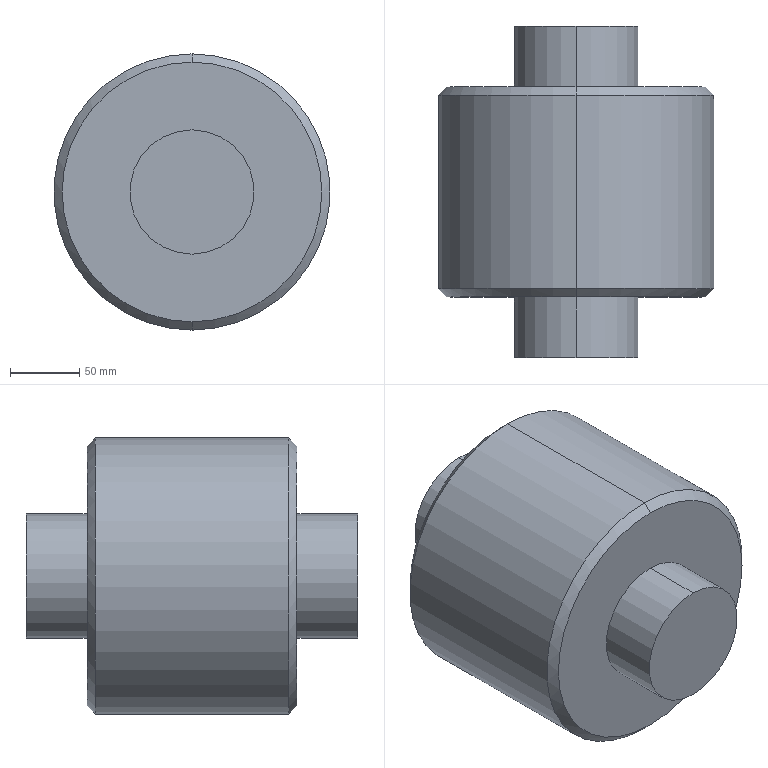Part | SolidWorks | features Chamfer 1, Extrusion 1, ICE 1 | 1 solid | 14 faces | box 200 x 240 x 200 mm | volume 5312886 mm3 | cylinder 6 | cone 4 | plane 4 | commonest cylinder face diameters 90 x4 200 x2
STEP:
#1=CARTESIAN_POINT('',(0.,196.,94.));
#2=VERTEX_POINT('',#1);
#3=CARTESIAN_POINT('',(0.,196.,-94.));
#4=VERTEX_POINT('',#3);
#5=CARTESIAN_POINT('',(0.,196.,0.));
#6=DIRECTION('',(0.,1.,0.));
#7=DIRECTION('',(0.,0.,1.));
#8=AXIS2_PLACEMENT_3D('',#5,#6,#7);
#9=CIRCLE('',#8,94.);
#10=EDGE_CURVE('',#2,#4,#9,.T.);
#11=ORIENTED_EDGE('',*,*,#10,.F.);
#12=CARTESIAN_POINT('',(0.,190.,100.));
#13=VERTEX_POINT('',#12);
#14=CARTESIAN_POINT('',(0.,196.,94.));
#15=DIRECTION('',(0.,-0.7071,0.7071));
#16=VECTOR('',#15,1000.);
#17=LINE('',#14,#16);
#18=EDGE_CURVE('',#2,#13,#17,.T.);
#19=ORIENTED_EDGE('',*,*,#18,.T.);
#20=CARTESIAN_POINT('',(0.,190.,-100.));
#21=VERTEX_POINT('',#20);
#22=CARTESIAN_POINT('',(0.,190.,0.));
#23=DIRECTION('',(0.,-1.,0.));
#24=DIRECTION('',(0.,0.,1.));
#25=AXIS2_PLACEMENT_3D('',#22,#23,#24);
#26=CIRCLE('',#25,100.);
#27=EDGE_CURVE('',#21,#13,#26,.T.);
#28=ORIENTED_EDGE('',*,*,#27,.F.);
#29=CARTESIAN_POINT('',(0.,196.,-94.));
#30=DIRECTION('',(0.,-0.7071,-0.7071));
#31=VECTOR('',#30,1000.);
#32=LINE('',#29,#31);
#33=EDGE_CURVE('',#4,#21,#32,.T.);
#34=ORIENTED_EDGE('',*,*,#33,.F.);
#35=EDGE_LOOP('',(#11,#19,#28,#34));
#36=FACE_OUTER_BOUND('',#35,.T.);
#37=CARTESIAN_POINT('',(0.,196.,0.));
#38=DIRECTION('',(0.,-1.,0.));
#39=DIRECTION('',(0.,0.,-1.));
#40=AXIS2_PLACEMENT_3D('',#37,#38,#39);
#41=CONICAL_SURFACE('',#40,94.,0.7854);
#42=ADVANCED_FACE('',(#36),#41,.T.);
#43=CARTESIAN_POINT('',(0.,44.,-94.));
#44=VERTEX_POINT('',#43);
#45=CARTESIAN_POINT('',(0.,44.,94.));
#46=VERTEX_POINT('',#45);
#47=CARTESIAN_POINT('',(0.,44.,0.));
#48=DIRECTION('',(0.,-1.,0.));
#49=DIRECTION('',(0.,0.,1.));
#50=AXIS2_PLACEMENT_3D('',#47,#48,#49);
#51=CIRCLE('',#50,94.);
#52=EDGE_CURVE('',#44,#46,#51,.T.);
#53=ORIENTED_EDGE('',*,*,#52,.F.);
#54=CARTESIAN_POINT('',(0.,50.,-100.));
#55=VERTEX_POINT('',#54);
#56=CARTESIAN_POINT('',(0.,50.,-100.));
#57=DIRECTION('',(0.,0.7071,-0.7071));
#58=VECTOR('',#57,1000.);
#59=LINE('',#56,#58);
#60=EDGE_CURVE('',#44,#55,#59,.T.);
#61=ORIENTED_EDGE('',*,*,#60,.T.);
#62=CARTESIAN_POINT('',(0.,50.,100.));
#63=VERTEX_POINT('',#62);
#64=CARTESIAN_POINT('',(0.,50.,0.));
#65=DIRECTION('',(0.,1.,0.));
#66=DIRECTION('',(0.,0.,1.));
#67=AXIS2_PLACEMENT_3D('',#64,#65,#66);
#68=CIRCLE('',#67,100.);
#69=EDGE_CURVE('',#63,#55,#68,.T.);
#70=ORIENTED_EDGE('',*,*,#69,.F.);
#71=CARTESIAN_POINT('',(0.,50.,100.));
#72=DIRECTION('',(0.,0.7071,0.7071));
#73=VECTOR('',#72,1000.);
#74=LINE('',#71,#73);
#75=EDGE_CURVE('',#46,#63,#74,.T.);
#76=ORIENTED_EDGE('',*,*,#75,.F.);
#77=EDGE_LOOP('',(#53,#61,#70,#76));
#78=FACE_OUTER_BOUND('',#77,.T.);
#79=CARTESIAN_POINT('',(0.,50.,0.));
#80=DIRECTION('',(0.,1.,0.));
#81=DIRECTION('',(0.,0.,1.));
#82=AXIS2_PLACEMENT_3D('',#79,#80,#81);
#83=CONICAL_SURFACE('',#82,100.,0.7854);
#84=ADVANCED_FACE('',(#78),#83,.T.);
#85=CARTESIAN_POINT('',(0.,240.,45.));
#86=VERTEX_POINT('',#85);
#87=CARTESIAN_POINT('',(0.,240.,-45.));
#88=VERTEX_POINT('',#87);
#89=CARTESIAN_POINT('',(0.,240.,0.));
#90=DIRECTION('',(0.,1.,0.));
#91=DIRECTION('',(0.,0.,1.));
#92=AXIS2_PLACEMENT_3D('',#89,#90,#91);
#93=CIRCLE('',#92,45.);
#94=EDGE_CURVE('',#86,#88,#93,.T.);
#95=ORIENTED_EDGE('',*,*,#94,.F.);
#96=CARTESIAN_POINT('',(0.,196.,45.));
#97=VERTEX_POINT('',#96);
#98=CARTESIAN_POINT('',(0.,240.,45.));
#99=DIRECTION('',(0.,-1.,0.));
#100=VECTOR('',#99,1000.);
#101=LINE('',#98,#100);
#102=EDGE_CURVE('',#86,#97,#101,.T.);
#103=ORIENTED_EDGE('',*,*,#102,.T.);
#104=CARTESIAN_POINT('',(0.,196.,-45.));
#105=VERTEX_POINT('',#104);
#106=CARTESIAN_POINT('',(0.,196.,0.));
#107=DIRECTION('',(0.,1.,0.));
#108=DIRECTION('',(0.,0.,1.));
#109=AXIS2_PLACEMENT_3D('',#106,#107,#108);
#110=CIRCLE('',#109,45.);
#111=EDGE_CURVE('',#97,#105,#110,.T.);
#112=ORIENTED_EDGE('',*,*,#111,.T.);
#113=CARTESIAN_POINT('',(0.,240.,-45.));
#114=DIRECTION('',(0.,-1.,0.));
#115=VECTOR('',#114,1000.);
#116=LINE('',#113,#115);
#117=EDGE_CURVE('',#88,#105,#116,.T.);
#118=ORIENTED_EDGE('',*,*,#117,.F.);
#119=EDGE_LOOP('',(#95,#103,#112,#118));
#120=FACE_OUTER_BOUND('',#119,.T.);
#121=CARTESIAN_POINT('',(0.,240.,0.));
#122=DIRECTION('',(0.,-1.,0.));
#123=DIRECTION('',(0.,0.,-1.));
#124=AXIS2_PLACEMENT_3D('',#121,#122,#123);
#125=CYLINDRICAL_SURFACE('',#124,45.);
#126=ADVANCED_FACE('',(#120),#125,.T.);
#127=ORIENTED_EDGE('',*,*,#69,.T.);
#128=CARTESIAN_POINT('',(0.,44.,-100.));
#129=DIRECTION('',(0.,1.,0.));
#130=VECTOR('',#129,1000.);
#131=LINE('',#128,#130);
#132=EDGE_CURVE('',#55,#21,#131,.T.);
#133=ORIENTED_EDGE('',*,*,#132,.T.);
#134=ORIENTED_EDGE('',*,*,#27,.T.);
#135=CARTESIAN_POINT('',(0.,44.,100.));
#136=DIRECTION('',(0.,1.,0.));
#137=VECTOR('',#136,1000.);
#138=LINE('',#135,#137);
#139=EDGE_CURVE('',#63,#13,#138,.T.);
#140=ORIENTED_EDGE('',*,*,#139,.F.);
#141=EDGE_LOOP('',(#127,#133,#134,#140));
#142=FACE_OUTER_BOUND('',#141,.T.);
#143=CARTESIAN_POINT('',(0.,44.,0.));
#144=DIRECTION('',(0.,1.,0.));
#145=DIRECTION('',(0.,0.,1.));
#146=AXIS2_PLACEMENT_3D('',#143,#144,#145);
#147=CYLINDRICAL_SURFACE('',#146,100.);
#148=ADVANCED_FACE('',(#142),#147,.T.);
#149=CARTESIAN_POINT('',(0.,44.,45.));
#150=VERTEX_POINT('',#149);
#151=CARTESIAN_POINT('',(0.,44.,-45.));
#152=VERTEX_POINT('',#151);
#153=CARTESIAN_POINT('',(0.,44.,0.));
#154=DIRECTION('',(0.,1.,0.));
#155=DIRECTION('',(0.,0.,1.));
#156=AXIS2_PLACEMENT_3D('',#153,#154,#155);
#157=CIRCLE('',#156,45.);
#158=EDGE_CURVE('',#150,#152,#157,.T.);
#159=ORIENTED_EDGE('',*,*,#158,.F.);
#160=CARTESIAN_POINT('',(0.,0.,45.));
#161=VERTEX_POINT('',#160);
#162=CARTESIAN_POINT('',(0.,240.,45.));
#163=DIRECTION('',(0.,-1.,0.));
#164=VECTOR('',#163,1000.);
#165=LINE('',#162,#164);
#166=EDGE_CURVE('',#150,#161,#165,.T.);
#167=ORIENTED_EDGE('',*,*,#166,.T.);
#168=CARTESIAN_POINT('',(0.,0.,-45.));
#169=VERTEX_POINT('',#168);
#170=CARTESIAN_POINT('',(0.,0.,0.));
#171=DIRECTION('',(0.,1.,0.));
#172=DIRECTION('',(0.,0.,1.));
#173=AXIS2_PLACEMENT_3D('',#170,#171,#172);
#174=CIRCLE('',#173,45.);
#175=EDGE_CURVE('',#161,#169,#174,.T.);
#176=ORIENTED_EDGE('',*,*,#175,.T.);
#177=CARTESIAN_POINT('',(0.,240.,-45.));
#178=DIRECTION('',(0.,-1.,0.));
#179=VECTOR('',#178,1000.);
#180=LINE('',#177,#179);
#181=EDGE_CURVE('',#152,#169,#180,.T.);
#182=ORIENTED_EDGE('',*,*,#181,.F.);
#183=EDGE_LOOP('',(#159,#167,#176,#182));
#184=FACE_OUTER_BOUND('',#183,.T.);
#185=CARTESIAN_POINT('',(0.,240.,0.));
#186=DIRECTION('',(0.,-1.,0.));
#187=DIRECTION('',(0.,0.,-1.));
#188=AXIS2_PLACEMENT_3D('',#185,#186,#187);
#189=CYLINDRICAL_SURFACE('',#188,45.);
#190=ADVANCED_FACE('',(#184),#189,.T.);
#191=ORIENTED_EDGE('',*,*,#166,.F.);
#192=CARTESIAN_POINT('',(0.,44.,0.));
#193=DIRECTION('',(0.,1.,0.));
#194=DIRECTION('',(0.,0.,1.));
#195=AXIS2_PLACEMENT_3D('',#192,#193,#194);
#196=CIRCLE('',#195,45.);
#197=EDGE_CURVE('',#152,#150,#196,.T.);
#198=ORIENTED_EDGE('',*,*,#197,.F.);
#199=ORIENTED_EDGE('',*,*,#181,.T.);
#200=CARTESIAN_POINT('',(0.,0.,0.));
#201=DIRECTION('',(0.,1.,0.));
#202=DIRECTION('',(0.,0.,1.));
#203=AXIS2_PLACEMENT_3D('',#200,#201,#202);
#204=CIRCLE('',#203,45.);
#205=EDGE_CURVE('',#169,#161,#204,.T.);
#206=ORIENTED_EDGE('',*,*,#205,.T.);
#207=EDGE_LOOP('',(#191,#198,#199,#206));
#208=FACE_OUTER_BOUND('',#207,.T.);
#209=CARTESIAN_POINT('',(0.,240.,0.));
#210=DIRECTION('',(0.,-1.,0.));
#211=DIRECTION('',(0.,0.,-1.));
#212=AXIS2_PLACEMENT_3D('',#209,#210,#211);
#213=CYLINDRICAL_SURFACE('',#212,45.);
#214=ADVANCED_FACE('',(#208),#213,.T.);
#215=ORIENTED_EDGE('',*,*,#205,.F.);
#216=ORIENTED_EDGE('',*,*,#175,.F.);
#217=EDGE_LOOP('',(#215,#216));
#218=FACE_OUTER_BOUND('',#217,.T.);
#219=CARTESIAN_POINT('',(0.,0.,0.));
#220=DIRECTION('',(0.,1.,0.));
#221=DIRECTION('',(0.,0.,1.));
#222=AXIS2_PLACEMENT_3D('',#219,#220,#221);
#223=PLANE('',#222);
#224=ADVANCED_FACE('',(#218),#223,.F.);
#225=ORIENTED_EDGE('',*,*,#132,.F.);
#226=CARTESIAN_POINT('',(0.,50.,0.));
#227=DIRECTION('',(0.,1.,0.));
#228=DIRECTION('',(0.,0.,1.));
#229=AXIS2_PLACEMENT_3D('',#226,#227,#228);
#230=CIRCLE('',#229,100.);
#231=EDGE_CURVE('',#55,#63,#230,.T.);
#232=ORIENTED_EDGE('',*,*,#231,.T.);
#233=ORIENTED_EDGE('',*,*,#139,.T.);
#234=CARTESIAN_POINT('',(0.,190.,0.));
#235=DIRECTION('',(0.,-1.,0.));
#236=DIRECTION('',(0.,0.,1.));
#237=AXIS2_PLACEMENT_3D('',#234,#235,#236);
#238=CIRCLE('',#237,100.);
#239=EDGE_CURVE('',#13,#21,#238,.T.);
#240=ORIENTED_EDGE('',*,*,#239,.T.);
#241=EDGE_LOOP('',(#225,#232,#233,#240));
#242=FACE_OUTER_BOUND('',#241,.T.);
#243=CARTESIAN_POINT('',(0.,44.,0.));
#244=DIRECTION('',(0.,1.,0.));
#245=DIRECTION('',(0.,0.,1.));
#246=AXIS2_PLACEMENT_3D('',#243,#244,#245);
#247=CYLINDRICAL_SURFACE('',#246,100.);
#248=ADVANCED_FACE('',(#242),#247,.T.);
#249=CARTESIAN_POINT('',(0.,44.,0.));
#250=DIRECTION('',(0.,-1.,0.));
#251=DIRECTION('',(0.,0.,1.));
#252=AXIS2_PLACEMENT_3D('',#249,#250,#251);
#253=CIRCLE('',#252,94.);
#254=EDGE_CURVE('',#46,#44,#253,.T.);
#255=ORIENTED_EDGE('',*,*,#254,.T.);
#256=ORIENTED_EDGE('',*,*,#52,.T.);
#257=EDGE_LOOP('',(#255,#256));
#258=FACE_OUTER_BOUND('',#257,.T.);
#259=ORIENTED_EDGE('',*,*,#197,.T.);
#260=ORIENTED_EDGE('',*,*,#158,.T.);
#261=EDGE_LOOP('',(#259,#260));
#262=FACE_BOUND('',#261,.T.);
#263=CARTESIAN_POINT('',(0.,44.,0.));
#264=DIRECTION('',(0.,1.,0.));
#265=DIRECTION('',(0.,0.,1.));
#266=AXIS2_PLACEMENT_3D('',#263,#264,#265);
#267=PLANE('',#266);
#268=ADVANCED_FACE('',(#258,#262),#267,.F.);
#269=CARTESIAN_POINT('',(0.,196.,0.));
#270=DIRECTION('',(0.,1.,0.));
#271=DIRECTION('',(0.,0.,1.));
#272=AXIS2_PLACEMENT_3D('',#269,#270,#271);
#273=CIRCLE('',#272,94.);
#274=EDGE_CURVE('',#4,#2,#273,.T.);
#275=ORIENTED_EDGE('',*,*,#274,.T.);
#276=ORIENTED_EDGE('',*,*,#10,.T.);
#277=EDGE_LOOP('',(#275,#276));
#278=FACE_OUTER_BOUND('',#277,.T.);
#279=CARTESIAN_POINT('',(0.,196.,0.));
#280=DIRECTION('',(0.,1.,0.));
#281=DIRECTION('',(0.,0.,1.));
#282=AXIS2_PLACEMENT_3D('',#279,#280,#281);
#283=CIRCLE('',#282,45.);
#284=EDGE_CURVE('',#105,#97,#283,.T.);
#285=ORIENTED_EDGE('',*,*,#284,.F.);
#286=ORIENTED_EDGE('',*,*,#111,.F.);
#287=EDGE_LOOP('',(#285,#286));
#288=FACE_BOUND('',#287,.T.);
#289=CARTESIAN_POINT('',(0.,196.,0.));
#290=DIRECTION('',(0.,1.,0.));
#291=DIRECTION('',(0.,0.,1.));
#292=AXIS2_PLACEMENT_3D('',#289,#290,#291);
#293=PLANE('',#292);
#294=ADVANCED_FACE('',(#278,#288),#293,.T.);
#295=CARTESIAN_POINT('',(0.,240.,0.));
#296=DIRECTION('',(0.,1.,0.));
#297=DIRECTION('',(0.,0.,1.));
#298=AXIS2_PLACEMENT_3D('',#295,#296,#297);
#299=CIRCLE('',#298,45.);
#300=EDGE_CURVE('',#88,#86,#299,.T.);
#301=ORIENTED_EDGE('',*,*,#300,.T.);
#302=ORIENTED_EDGE('',*,*,#94,.T.);
#303=EDGE_LOOP('',(#301,#302));
#304=FACE_OUTER_BOUND('',#303,.T.);
#305=CARTESIAN_POINT('',(0.,240.,0.));
#306=DIRECTION('',(0.,1.,0.));
#307=DIRECTION('',(0.,0.,1.));
#308=AXIS2_PLACEMENT_3D('',#305,#306,#307);
#309=PLANE('',#308);
#310=ADVANCED_FACE('',(#304),#309,.T.);
#311=ORIENTED_EDGE('',*,*,#102,.F.);
#312=ORIENTED_EDGE('',*,*,#300,.F.);
#313=ORIENTED_EDGE('',*,*,#117,.T.);
#314=ORIENTED_EDGE('',*,*,#284,.T.);
#315=EDGE_LOOP('',(#311,#312,#313,#314));
#316=FACE_OUTER_BOUND('',#315,.T.);
#317=CARTESIAN_POINT('',(0.,240.,0.));
#318=DIRECTION('',(0.,-1.,0.));
#319=DIRECTION('',(0.,0.,-1.));
#320=AXIS2_PLACEMENT_3D('',#317,#318,#319);
#321=CYLINDRICAL_SURFACE('',#320,45.);
#322=ADVANCED_FACE('',(#316),#321,.T.);
#323=ORIENTED_EDGE('',*,*,#60,.F.);
#324=ORIENTED_EDGE('',*,*,#254,.F.);
#325=ORIENTED_EDGE('',*,*,#75,.T.);
#326=ORIENTED_EDGE('',*,*,#231,.F.);
#327=EDGE_LOOP('',(#323,#324,#325,#326));
#328=FACE_OUTER_BOUND('',#327,.T.);
#329=CARTESIAN_POINT('',(0.,50.,0.));
#330=DIRECTION('',(0.,1.,0.));
#331=DIRECTION('',(0.,0.,1.));
#332=AXIS2_PLACEMENT_3D('',#329,#330,#331);
#333=CONICAL_SURFACE('',#332,100.,0.7854);
#334=ADVANCED_FACE('',(#328),#333,.T.);
#335=ORIENTED_EDGE('',*,*,#18,.F.);
#336=ORIENTED_EDGE('',*,*,#274,.F.);
#337=ORIENTED_EDGE('',*,*,#33,.T.);
#338=ORIENTED_EDGE('',*,*,#239,.F.);
#339=EDGE_LOOP('',(#335,#336,#337,#338));
#340=FACE_OUTER_BOUND('',#339,.T.);
#341=CARTESIAN_POINT('',(0.,196.,0.));
#342=DIRECTION('',(0.,-1.,0.));
#343=DIRECTION('',(0.,0.,-1.));
#344=AXIS2_PLACEMENT_3D('',#341,#342,#343);
#345=CONICAL_SURFACE('',#344,94.,0.7854);
#346=ADVANCED_FACE('',(#340),#345,.T.);
#347=CLOSED_SHELL('',(#42,#84,#126,#148,#190,#214,#224,#248,#268,#294,#310,#322,#334,#346));
#348=MANIFOLD_SOLID_BREP('',#347);
#349=CARTESIAN_POINT('',(0.,0.,0.));
#350=DIRECTION('',(0.,0.,1.));
#351=DIRECTION('',(1.,0.,0.));
#352=AXIS2_PLACEMENT_3D('',#349,#350,#351);
#353=(LENGTH_UNIT()NAMED_UNIT(*)SI_UNIT(.MILLI.,.METRE.));
#354=UNCERTAINTY_MEASURE_WITH_UNIT(LENGTH_MEASURE(0.00001),#353,'','');
#355=(NAMED_UNIT(*)PLANE_ANGLE_UNIT()SI_UNIT($,.RADIAN.));
#356=(NAMED_UNIT(*)SI_UNIT($,.STERADIAN.)SOLID_ANGLE_UNIT());
#357=(GEOMETRIC_REPRESENTATION_CONTEXT(3)GLOBAL_UNCERTAINTY_ASSIGNED_CONTEXT((#354))GLOBAL_UNIT_ASSIGNED_CONTEXT((#353,#355,#356))REPRESENTATION_CONTEXT('',''));
#358=ADVANCED_BREP_SHAPE_REPRESENTATION('',(#348,#352),#357);